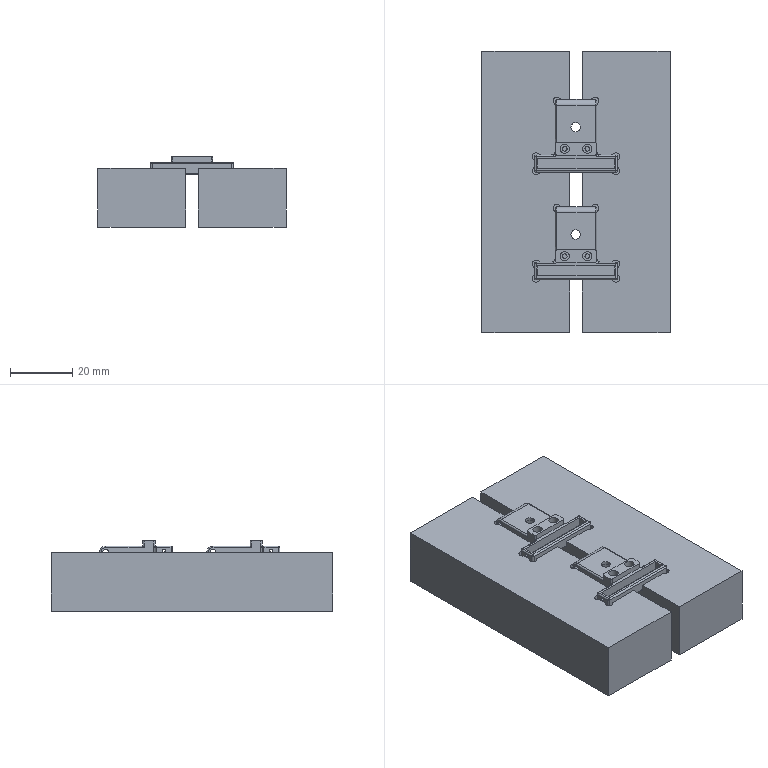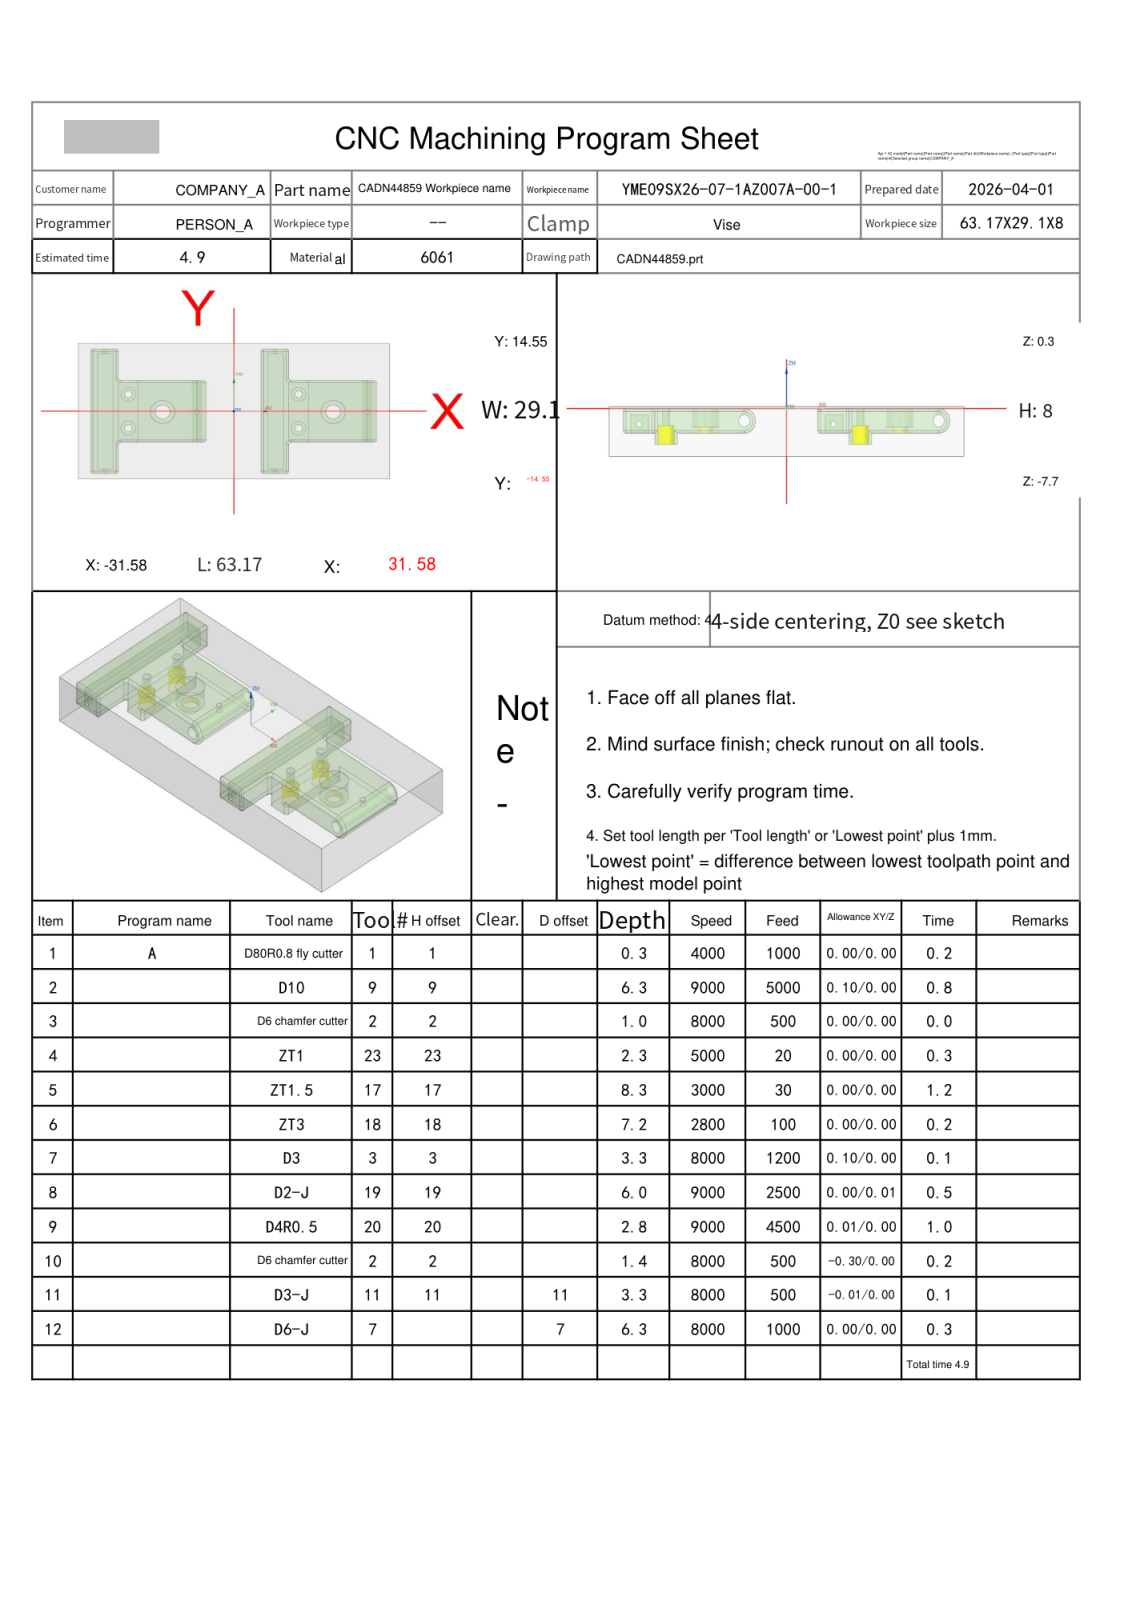NC program | NX | posted by the shop | part box 60.696 x 90.669 x 22.754 mm
Lines 2495 to 3978 of 3978:
N9 T20 M06
(D4R0.5  D=4. R=0.5 H=20 ce=0.01 di=0.00)
G00 G90 G54 X-3.173 Y-7.756 M03 S9000
G43 H20 Z10.3
M08
Z.484
G01 Z-.016 F4500.
X-6.415 Y-7.798
X-7.496 Y-7.812
X-7.515 Y-7.821
X-22.266
Y-12.848
G02 X-23.952 Y-14.535 I-1.687 J0.0
G01 X-28.584
G02 X-30.271 Y-12.848 I0.0 J1.687
G01 Y12.848
G02 X-28.584 Y14.535 I1.687 J0.0
G01 X-23.952
G02 X-22.266 Y12.848 I0.0 J-1.687
G01 Y7.821
X-7.515
X-7.496 Y7.812
X-6.415 Y7.798
Y7.852 Z-.028
Y7.904 Z-.04
X-7.515 Y7.925
X-22.162
Y12.848
G03 X-23.952 Y14.639 I-1.791 J0.0
G01 X-28.584
G03 X-30.375 Y12.848 I0.0 J-1.791
G01 Y-12.848
G03 X-28.584 Y-14.639 I1.791 J0.0
G01 X-23.952
G03 X-22.162 Y-12.848 I0.0 J1.791
G01 Y-7.925
X-7.515
X-6.415 Y-7.904
Y-7.963 Z-.057
Y-8.002 Z-.074
X-7.496 Y-8.013
X-7.515 Y-8.02
X-22.066
Y-12.848
G02 X-23.952 Y-14.734 I-1.886 J0.0
G01 X-28.584
G02 X-30.471 Y-12.848 I0.0 J1.886
G01 Y12.848
G02 X-28.584 Y14.734 I1.886 J0.0
G01 X-23.952
G02 X-22.066 Y12.848 I0.0 J-1.886
G01 Y8.02
X-7.515
X-7.496 Y8.013
X-6.415 Y8.002
Y8.055 Z-.095
Y8.101 Z-.116
X-7.496 Y8.106
X-7.515 Y8.112
X-21.974
Y12.848
G03 X-23.952 Y14.826 I-1.978 J0.0
G01 X-28.584
G03 X-30.562 Y12.848 I0.0 J-1.978
G01 Y-12.848
G03 X-28.584 Y-14.826 I1.978 J0.0
G01 X-23.952
G03 X-21.974 Y-12.848 I0.0 J1.978
G01 Y-8.112
X-7.515
X-7.496 Y-8.106
X-6.415 Y-8.101
Y-8.151 Z-.142
X-6.416 Y-8.191 Z-.168
X-7.496 Y-8.196
X-7.515 Y-8.198
X-21.888
Y-12.848
G02 X-23.952 Y-14.913 I-2.065 J0.0
G01 X-28.584
G02 X-30.649 Y-12.848 I0.0 J2.065
G01 Y12.848
G02 X-28.584 Y14.913 I2.065 J0.0
G01 X-23.952
G02 X-21.888 Y12.848 I0.0 J-2.065
G01 Y8.198
X-7.515
X-7.496 Y8.196
X-6.416 Y8.191
X-6.415 Y8.236 Z-.198
Y8.273 Z-.228
X-7.496
X-7.515 Y8.279
X-21.807
Y12.848
G03 X-23.952 Y14.994 I-2.146 J0.0
G01 X-28.584
G03 X-30.73 Y12.848 I0.0 J-2.146
G01 Y-12.848
G03 X-28.584 Y-14.994 I2.146 J0.0
G01 X-23.952
G03 X-21.807 Y-12.848 I0.0 J2.146
G01 Y-8.279
X-7.515
X-7.496 Y-8.273
X-6.415
Y-8.31 Z-.262
Y-8.351 Z-.296
X-7.515 Y-8.354
X-21.732
Y-12.848
G02 X-23.952 Y-15.068 I-2.22 J0.0
G01 X-28.584
G02 X-30.804 Y-12.848 I0.0 J2.22
G01 Y12.848
G02 X-28.584 Y15.068 I2.22 J0.0
G01 X-23.952
G02 X-21.732 Y12.848 I0.0 J-2.22
G01 Y8.354
X-7.515
X-6.415 Y8.351
Y8.385 Z-.333
X-6.416 Y8.415 Z-.37
X-7.496 Y8.412
X-7.515 Y8.421
X-21.665
Y12.848
G03 X-23.952 Y15.135 I-2.287 J0.0
G01 X-28.584
G03 X-30.871 Y12.848 I0.0 J-2.287
G01 Y-12.848
G03 X-28.584 Y-15.135 I2.287 J0.0
G01 X-23.952
G03 X-21.665 Y-12.848 I0.0 J2.287
G01 Y-8.421
X-7.515
X-7.496 Y-8.412
X-6.416 Y-8.415
X-6.415 Y-8.448 Z-.411
Y-8.476 Z-.451
X-7.496
X-7.515 Y-8.48
X-21.606
Y-12.848
G02 X-23.952 Y-15.194 I-2.346 J0.0
G01 X-28.584
G02 X-30.931 Y-12.848 I0.0 J2.346
G01 Y12.848
G02 X-28.584 Y15.194 I2.346 J0.0
G01 X-23.952
G02 X-21.606 Y12.848 I0.0 J-2.346
G01 Y8.48
X-7.515
X-7.496 Y8.476
X-6.415
Y8.5 Z-.495
Y8.526 Z-.538
X-7.496 Y8.527
X-7.515 Y8.531
X-21.556
Y12.848
G03 X-23.952 Y15.245 I-2.397 J0.0
G01 X-28.584
G03 X-30.981 Y12.848 I0.0 J-2.397
G01 Y-12.848
G03 X-28.584 Y-15.245 I2.397 J0.0
G01 X-23.952
G03 X-21.556 Y-12.848 I0.0 J2.397
G01 Y-8.531
X-7.515
X-7.496 Y-8.527
X-6.424 Y-8.525
Y-8.544 Z-.583
Y-8.57 Z-.629
X-7.515 Y-8.572
X-21.514
Y-12.848
G02 X-23.952 Y-15.287 I-2.439 J0.0
G01 X-28.584
G02 X-31.023 Y-12.848 I0.0 J2.439
G01 Y12.848
G02 X-28.584 Y15.287 I2.439 J0.0
G01 X-23.952
G02 X-21.514 Y12.848 I0.0 J-2.439
G01 Y8.572
X-7.515
X-6.415 Y8.567
Y8.586 Z-.675
Y8.599 Z-.722
X-7.515 Y8.604
X-21.482
Y12.848
G03 X-23.952 Y15.318 I-2.47 J0.0
G01 X-28.584
G03 X-31.055 Y12.848 I0.0 J-2.47
G01 Y-12.848
G03 X-28.584 Y-15.318 I2.47 J0.0
G01 X-23.952
G03 X-21.482 Y-12.848 I0.0 J2.47
G01 Y-8.604
X-7.515
X-6.424 Y-8.6
Y-8.613 Z-.768
Y-8.625 Z-.814
X-7.515 Y-8.626
X-21.46
Y-12.848
G02 X-23.952 Y-15.341 I-2.493 J0.0
G01 X-28.584
G02 X-31.077 Y-12.848 I0.0 J2.493
G01 Y12.848
G02 X-28.584 Y15.341 I2.493 J0.0
G01 X-23.952
G02 X-21.46 Y12.848 I0.0 J-2.493
G01 Y8.626
X-7.515
X-6.424 Y8.622
Y8.629 Z-.861
Y8.634 Z-.907
X-6.433 Y8.633
X-7.496 Y8.636
X-7.515 Y8.64
X-21.447
Y12.848
G03 X-23.952 Y15.354 I-2.506 J0.0
G01 X-28.584
G03 X-31.09 Y12.848 I0.0 J-2.506
G01 Y-12.848
G03 X-28.584 Y-15.354 I2.506 J0.0
G01 X-23.952
G03 X-21.447 Y-12.848 I0.0 J2.506
G01 Y-8.64
X-7.515
X-7.496 Y-8.636
X-6.424 Y-8.635
Y-8.643 Z-1.
X-7.515 Y-8.644
X-21.387
X-21.442
Y-8.779
Y-12.858
X-21.446 Y-12.978
G02 X-23.655 Y-15.34 I-2.507 J.13
G01 X-23.952 Y-15.358
X-28.595 Y-15.357
X-28.724 Y-15.354
G02 X-31.094 Y-12.848 I.139 J2.506
G01 Y12.858
X-31.088 Y13.027
G02 X-28.724 Y15.354 I2.504 J-.179
G01 X-28.585 Y15.358
X-23.952
X-23.655 Y15.34
G02 X-21.442 Y12.848 I-.297 J-2.492
G01 Y8.779
Y8.644
X-21.387
X-7.515
X-6.424 Y8.643
G00 Z10.3
X31.436 Y-7.732
Z.484
G01 Z-.016
X28.185 Y-7.798
X27.085 Y-7.821
X12.334
Y-12.848
G02 X10.648 Y-14.535 I-1.687 J0.0
G01 X6.016
G02 X4.329 Y-12.848 I0.0 J1.687
G01 Y12.848
G02 X6.016 Y14.535 I1.687 J0.0
G01 X10.648
G02 X12.334 Y12.848 I0.0 J-1.687
G01 Y7.821
X27.085
X28.185 Y7.798
Y7.852 Z-.028
Y7.904 Z-.04
X27.085 Y7.925
X12.438
Y12.848
G03 X10.648 Y14.639 I-1.791 J0.0
G01 X6.016
G03 X4.225 Y12.848 I0.0 J-1.791
G01 Y-12.848
G03 X6.016 Y-14.639 I1.791 J0.0
G01 X10.648
G03 X12.438 Y-12.848 I0.0 J1.791
G01 Y-7.925
X27.085
X28.185 Y-7.904
Y-7.962 Z-.057
Y-8.003 Z-.074
X27.085 Y-8.02
X12.534
Y-12.848
G02 X10.648 Y-14.734 I-1.886 J0.0
G01 X6.016
G02 X4.129 Y-12.848 I0.0 J1.886
G01 Y12.848
G02 X6.016 Y14.734 I1.886 J0.0
G01 X10.648
G02 X12.534 Y12.848 I0.0 J-1.886
G01 Y8.02
X27.085
X28.185 Y8.003
Y8.055 Z-.095
Y8.101 Z-.116
X27.085 Y8.112
X12.626
Y12.848
G03 X10.648 Y14.826 I-1.978 J0.0
G01 X6.016
G03 X4.038 Y12.848 I0.0 J-1.978
G01 Y-12.848
G03 X6.016 Y-14.826 I1.978 J0.0
G01 X10.648
G03 X12.626 Y-12.848 I0.0 J1.978
G01 Y-8.112
X27.085
X28.185 Y-8.101
Y-8.148 Z-.142
Y-8.191 Z-.168
X27.085 Y-8.198
X12.712
Y-12.848
G02 X10.648 Y-14.913 I-2.065 J0.0
G01 X6.016
G02 X3.951 Y-12.848 I0.0 J2.065
G01 Y12.848
G02 X6.016 Y14.913 I2.065 J0.0
G01 X10.648
G02 X12.712 Y12.848 I0.0 J-2.065
G01 Y8.198
X27.085
X28.185 Y8.191
Y8.236 Z-.198
X28.184 Y8.272 Z-.228
X27.085 Y8.279
X12.793
Y12.848
G03 X10.648 Y14.994 I-2.146 J0.0
G01 X6.016
G03 X3.87 Y12.848 I0.0 J-2.146
G01 Y-12.848
G03 X6.016 Y-14.994 I2.146 J0.0
G01 X10.648
G03 X12.793 Y-12.848 I0.0 J2.146
G01 Y-8.279
X27.085
X28.184 Y-8.272
Y-8.314 Z-.262
Y-8.347 Z-.296
X28.154 Y-8.346
X27.085 Y-8.354
X12.868
Y-12.848
G02 X10.648 Y-15.068 I-2.22 J0.0
G01 X6.016
G02 X3.796 Y-12.848 I0.0 J2.22
G01 Y12.848
G02 X6.016 Y15.068 I2.22 J0.0
G01 X10.648
G02 X12.868 Y12.848 I0.0 J-2.22
G01 Y8.354
X27.085
X28.154 Y8.346
X28.184 Y8.347
Y8.381 Z-.333
Y8.415 Z-.37
X28.131
G02 X27.085 Y8.421 I0.0 J88.093
G01 X12.935
Y12.848
G03 X10.648 Y15.135 I-2.287 J0.0
G01 X6.016
G03 X3.729 Y12.848 I0.0 J-2.287
G01 Y-12.848
G03 X6.016 Y-15.135 I2.287 J0.0
G01 X10.648
G03 X12.935 Y-12.848 I0.0 J2.287
G01 Y-8.421
X27.085
G02 X27.747 Y-8.41 I.663 J-20.048
X28.184 Y-8.415 I0.0 J-20.059
G01 Y-8.445 Z-.411
Y-8.474 Z-.451
X27.085 Y-8.48
X12.994
Y-12.848
G02 X10.648 Y-15.194 I-2.346 J0.0
G01 X6.016
G02 X3.669 Y-12.848 I0.0 J2.346
G01 Y12.848
G02 X6.016 Y15.194 I2.346 J0.0
G01 X10.648
G02 X12.994 Y12.848 I0.0 J-2.346
G01 Y8.48
X27.085
X28.184 Y8.474
Y8.5 Z-.495
Y8.526 Z-.538
X27.085 Y8.531
X13.044
Y12.848
G03 X10.648 Y15.245 I-2.397 J0.0
G01 X6.016
G03 X3.619 Y12.848 I0.0 J-2.397
G01 Y-12.848
G03 X6.016 Y-15.245 I2.397 J0.0
G01 X10.648
G03 X13.044 Y-12.848 I0.0 J2.397
G01 Y-8.531
X27.085
X28.181 Y-8.525
Y-8.544 Z-.583
Y-8.57 Z-.629
X27.085 Y-8.572
X13.086
Y-12.848
G02 X10.648 Y-15.287 I-2.439 J0.0
G01 X6.016
G02 X3.577 Y-12.848 I0.0 J2.439
G01 Y12.848
G02 X6.016 Y15.287 I2.439 J0.0
G01 X10.648
G02 X13.086 Y12.848 I0.0 J-2.439
G01 Y8.572
X27.085
X28.184 Y8.567
Y8.586 Z-.675
Y8.599 Z-.722
X27.085 Y8.604
X13.118
Y12.848
G03 X10.648 Y15.318 I-2.47 J0.0
G01 X6.016
G03 X3.545 Y12.848 I0.0 J-2.47
G01 Y-12.848
G03 X6.016 Y-15.318 I2.47 J0.0
G01 X10.648
G03 X13.118 Y-12.848 I0.0 J2.47
G01 Y-8.604
X27.085
X28.181 Y-8.6
Y-8.613 Z-.768
Y-8.625 Z-.814
X27.085 Y-8.626
X13.14
Y-12.848
G02 X10.648 Y-15.341 I-2.493 J0.0
G01 X6.016
G02 X3.523 Y-12.848 I0.0 J2.493
G01 Y12.848
G02 X6.016 Y15.341 I2.493 J0.0
G01 X10.648
G02 X13.14 Y12.848 I0.0 J-2.493
G01 Y8.626
X27.085
X28.181 Y8.622
Y8.629 Z-.861
Y8.634 Z-.907
X28.172 Y8.633
X27.085 Y8.64
X13.153
Y12.848
G03 X10.648 Y15.354 I-2.506 J0.0
G01 X6.016
G03 X3.51 Y12.848 I0.0 J-2.506
G01 Y-12.848
G03 X6.016 Y-15.354 I2.506 J0.0
G01 X10.648
G03 X13.153 Y-12.848 I0.0 J2.506
G01 Y-8.64
X27.085
X28.181 Y-8.635
Y-8.643 Z-1.
X27.085 Y-8.644
X13.158
Y-12.848
G02 X10.804 Y-15.353 I-2.51 J0.0
G01 X10.648 Y-15.358
X6.015
X5.864 Y-15.353
G02 X3.509 Y-12.974 I.152 J2.505
G01 X3.506 Y-12.848
X3.507 Y12.858
X3.509 Y12.974
G02 X5.391 Y15.279 I2.507 J-.126
G01 X5.449 Y15.293
X5.68 Y15.335
X5.7 Y15.338
X5.864 Y15.353
X6.015 Y15.358
X10.648
X10.804 Y15.353
G02 X13.158 Y12.848 I-.156 J-2.505
G01 Y8.644
X27.085
X28.181 Y8.643
G00 Z10.3
G00 G90 X23.972 Y9.673 M03 S9000
Z10.3
Z.491
G01 Z-.009 F4500.
G03 X25.972 Y7.673 I2. J0.0
G02 X26.537 Y7.748 I.565 J-2.104
X28.641 Y6.134 I0.0 J-2.178
G01 Y-6.134
G02 X26.537 Y-7.748 I-2.104 J.565
X25.972 Y-7.673 I0.0 J2.178
G01 Y-7.815 Z-.015
Y-7.847 Z-.021
X27.135 Y-7.833
G03 X28.916 Y-6.134 I-.022 J1.806
G01 Y6.134
G03 X27.135 Y7.833 I-1.803 J-.107
G01 X25.972 Y7.847
Y7.883 Z-.029
Y7.898 Z-.037
X27.347 Y7.868
X27.555 Y7.824
G02 X28.999 Y6.134 I-.377 J-1.784
G01 Y-6.134
G02 X27.555 Y-7.824 I-1.821 J.094
G01 X27.347 Y-7.868
X25.972 Y-7.898
Y-7.947 Z-.047
Y-7.977 Z-.057
X27.263 Y-7.952
G03 X29.126 Y-6.134 I-.038 J1.903
G01 Y6.134
G03 X27.263 Y7.952 I-1.901 J-.085
G01 X25.972 Y7.977
Y8.01 Z-.069
Y8.039 Z-.081
X27.347 Y8.013
X27.63 Y7.966
G02 X29.227 Y6.134 I-.373 J-1.937
G01 Y-6.134
G02 X27.63 Y-7.966 I-1.969 J.105
G01 X27.347 Y-8.013
X25.972 Y-8.039
Y-8.07 Z-.095
Y-8.098 Z-.109
X27.347 Y-8.076
X27.566 Y-8.044
G03 X29.326 Y-6.134 I-.291 J2.033
G01 Y6.134
G03 X27.566 Y8.044 I-2.05 J-.122
G01 X27.347 Y8.076
X25.972 Y8.098
Y8.128 Z-.125
Y8.156 Z-.141
G02 X26.507 Y8.177 I.535 J-6.848
X27.805 Y8.053 I0.0 J-6.869
X29.422 Y6.134 I-.441 J-2.013
G01 Y-6.134
G02 X27.805 Y-8.053 I-2.058 J.093
X26.507 Y-8.177 I-1.298 J6.746
X25.972 Y-8.156 I0.0 J6.869
G01 Y-8.185 Z-.159
Y-8.211 Z-.177
X27.347 Y-8.197
X27.63 Y-8.155
G03 X29.518 Y-6.134 I-.298 J2.17
G01 Y6.134
G03 X27.63 Y8.155 I-2.185 J-.148
G01 X27.347 Y8.197
X25.972 Y8.211
Y8.239 Z-.196
Y8.265 Z-.216
X27.347 Y8.245
X27.551 Y8.222
G02 X29.052 Y7.488 I-.281 J-2.475
X29.611 Y6.134 I-1.568 J-1.439
G01 Y-6.134
G02 X28.48 Y-7.926 I-2.113 J.08
X27.11 Y-8.258 I-1.37 J2.66
G01 X27.064
X25.986
X25.972 Y-8.265
Y-8.291 Z-.237
Y-8.315 Z-.259
X27.245 Y-8.3
G03 X28.759 Y-7.832 I-.034 J2.79
X29.702 Y-6.134 I-1.176 J1.764
G01 Y6.139
G03 X29.364 Y7.219 I-1.892 J0.0
X27.63 Y8.264 I-2.033 J-1.413
G01 X27.347 Y8.299
X25.972 Y8.315
Y8.34 Z-.282
Y8.363 Z-.305
X27.347 Y8.349
X27.63 Y8.318
G02 X29.33 Y7.401 I-.3 J-2.588
X29.792 Y6.134 I-1.523 J-1.273
G01 Y-6.134
G02 X28.51 Y-8.053 I-2.204 J.084
X27.107 Y-8.359 I-1.403 J3.067
G01 X27.064
X25.986
X25.972 Y-8.363
Y-8.386 Z-.33
Y-8.408 Z-.355
X27.246 Y-8.392
G03 X28.76 Y-7.984 I-.04 J3.156
X29.879 Y-6.134 I-1.085 J1.92
G01 Y6.134
G03 X29.047 Y7.788 I-2.19 J-.065
X27.347 Y8.391 I-1.796 J-2.367
G01 X25.972 Y8.408
Y8.43 Z-.382
Y8.45 Z-.409
X27.347 Y8.435
X27.63 Y8.406
G02 X29.047 Y7.875 I-.296 J-2.94
X29.964 Y6.134 I-1.312 J-1.804
G01 Y-6.134
G02 X29.047 Y-7.875 I-2.23 J.063
X27.63 Y-8.406 I-1.712 J2.408
G01 X27.347 Y-8.435
X25.972 Y-8.45
Y-8.47 Z-.437
X25.973 Y-8.489 Z-.465
X27.347 Y-8.481
X27.63 Y-8.452
G03 X29.047 Y-7.95 I-.321 J3.157
X30.047 Y-6.134 I-1.248 J1.872
G01 Y6.134
G03 X29.047 Y7.95 I-2.249 J-.056
X27.63 Y8.452 I-1.738 J-2.656
G01 X27.347 Y8.481
X25.973 Y8.489
Y8.507 Z-.495
Y8.524 Z-.525
X27.347 Y8.514
X27.63 Y8.492
G02 X29.047 Y8.018 I-.296 J-3.237
X30.128 Y6.134 I-1.198 J-1.94
G01 Y-6.134
G02 X29.047 Y-8.018 I-2.279 J.056
X27.63 Y-8.492 I-1.712 J2.763
X26.493 Y-8.533 I-1.138 J15.871
X25.973 Y-8.524 I0.0 J15.911
G01 Y-8.54 Z-.557
Y-8.555 Z-.589
X27.347 Y-8.548
X27.63 Y-8.525
G03 X29.047 Y-8.082 I-.268 J3.342
X30.206 Y-6.134 I-1.149 J2.003
G01 Y6.134
G03 X29.047 Y8.082 I-2.309 J-.055
X27.63 Y8.525 I-1.684 J-2.899
G01 X27.347 Y8.548
X25.973 Y8.555
Y8.582 Z-.655
X25.987 Y8.576
X27.347 Y8.571
X27.63 Y8.555
G02 X29.047 Y8.143 I-.237 J-3.451
X30.281 Y6.134 I-1.112 J-2.067
G01 Y-6.134
G02 X29.047 Y-8.143 I-2.346 J.058
X27.63 Y-8.555 I-1.653 J3.038
G01 X27.347 Y-8.571
X25.987 Y-8.576
X25.973 Y-8.582
Y-8.594 Z-.689
Y-8.605 Z-.724
G03 X26.441 Y-8.61 I.468 J21.709
X27.63 Y-8.577 I0.0 J21.714
X29.047 Y-8.203 I-.173 J3.518
X30.354 Y-6.134 I-1.077 J2.128
G01 Y6.134
G03 X29.047 Y8.203 I-2.384 J-.059
X27.63 Y8.577 I-1.589 J-3.143
G01 X27.347 Y8.594
X25.973 Y8.605
X25.984 Y8.623 Z-.796
X27.352 Y8.618
X27.63 Y8.601
G02 X28.859 Y8.336 I-.17 J-3.771
X30.424 Y6.134 I-.869 J-2.274
G01 Y-6.134
G02 X28.859 Y-8.336 I-2.434 J.073
X27.63 Y-8.601 I-1.399 J3.506
G01 X27.352 Y-8.618
X25.984 Y-8.623
Y-8.635 Z-.871
X26.002 Y-8.63
X27.272
G03 X28.213 Y-8.555 I0.0 J5.964
X29.33 Y-8.141 I-.481 J3.007
G01 X29.471 Y-8.053
G03 X30.491 Y-6.134 I-1.377 J1.962
G01 Y6.134
G03 X30.041 Y7.488 I-2.364 J-.034
X28.674 Y8.443 I-2.109 J-1.564
X27.394 Y8.628 I-1.28 J-4.339
G01 X27.347 Y8.627
X26.002 Y8.63
X25.984 Y8.635
Y8.642 Z-.948
X27.347 Y8.636
X27.63 Y8.629
G02 X28.763 Y8.449 I-.065 J-4.068
X30.286 Y7.205 I-.762 J-2.488
X30.554 Y6.134 I-2.188 J-1.116
G01 Y-6.134
G02 X29.876 Y-7.771 I-2.394 J.034
X28.48 Y-8.526 I-1.964 J1.96
X27.898 Y-8.618 I-1.417 J7.085
X26.45 Y-8.645 I-1.448 J38.753
X25.984 Y-8.642 I0.0 J38.78
G01 X25.993 Y-8.644 Z-1.028
G03 X26.566 Y-8.648 I.573 J39.735
X27.914 Y-8.625 I0.0 J39.739
X29.625 Y-8.053 I-.089 J3.114
X30.615 Y-6.134 I-1.434 J1.954
G01 Y6.134
G03 X29.625 Y8.053 I-2.423 J-.035
X27.914 Y8.625 I-1.801 J-2.542
X26.678 Y8.652 I-1.235 J-28.393
X25.993 Y8.644 I0.0 J-28.42
G01 Z-1.11
X27.63
X28.022 Y8.629
G02 X29.613 Y8.113 I-.121 J-3.087
X30.672 Y6.134 I-1.395 J-2.02
G01 Y-6.134
G02 X29.613 Y-8.113 I-2.454 J.04
X28.023 Y-8.628 I-1.711 J2.57
G01 X27.63 Y-8.644
X25.993
Z-1.194
X27.63
X27.914 Y-8.641
G03 X29.304 Y-8.336 I0.0 J3.322
X30.726 Y-6.134 I-1.059 J2.244
G01 Y6.134
G03 X29.304 Y8.336 I-2.481 J-.042
X27.914 Y8.641 I-1.391 J-3.018
G01 X27.63 Y8.644
X25.993
Z-1.281
X27.914
X28.197 Y8.631
G02 X29.613 Y8.198 I-.099 J-2.86
X30.777 Y6.134 I-1.315 J-2.102
G01 Y-6.134
G02 X29.047 Y-8.471 I-2.517 J.054
X27.95 Y-8.644 I-1.096 J3.395
G01 X27.914
X25.993
Z-1.369
X28.033
G03 X29.059 Y-8.487 I0.0 J3.444
X30.766 Y-6.64 I-.752 J2.407
X30.824 Y-6.134 I-5.478 J.882
G01 Y6.134
G03 X30.766 Y6.64 I-5.536 J-.375
X29.613 Y8.235 I-2.436 J-.547
X28.197 Y8.637 I-1.472 J-2.488
G01 X27.914 Y8.644
X25.993
Z-1.459
X28.197
G02 X29.33 Y8.408 I-.03 J-2.989
X30.867 Y6.134 I-.963 J-2.308
G01 Y-6.134
G02 X29.33 Y-8.408 I-2.501 J.034
X28.197 Y-8.644 I-1.163 J2.754
G01 X25.993
Z-1.551
X28.197
X28.218
G03 X29.33 Y-8.435 I0.0 J3.061
X30.907 Y-6.134 I-.939 J2.335
G01 Y6.134
G03 X29.33 Y8.435 I-2.516 J-.034
X28.218 Y8.644 I-1.112 J-2.852
G01 X28.197
X25.993
Z-1.644
X28.197
X28.48 Y8.632
G02 X30.694 Y7.205 I-.091 J-2.573
X30.943 Y6.134 I-2.386 J-1.119
G01 Y-6.134
G02 X29.33 Y-8.453 I-2.508 J.023
X28.266 Y-8.645 I-1.063 J2.862
G01 X28.197 Y-8.644
X25.993
Z-1.739
X28.197
X28.48 Y-8.637
G03 X30.976 Y-6.134 I-.04 J2.535
G01 Y6.134
G03 X28.48 Y8.637 I-2.535 J-.032
G01 X28.197 Y8.644
X25.993
Z-1.835
X28.197
X28.48 Y8.641
G02 X31.004 Y6.134 I-.012 J-2.537
G01 Y-6.134
G02 X28.48 Y-8.641 I-2.537 J.029
G01 X28.197 Y-8.644
X25.993
Z-1.932
X28.48
X28.493
G03 X31.029 Y-6.134 I0.0 J2.536
G01 Y6.134
G03 X28.493 Y8.644 I-2.536 J-.026
G01 X28.48
X25.993
Z-2.03
X28.48
X28.507
G02 X30.805 Y7.205 I0.0 J-2.555
X31.05 Y6.134 I-2.318 J-1.093
G01 Y-6.134
G02 X28.864 Y-8.618 I-2.527 J.02
G01 X28.48 Y-8.644
X25.993
Z-2.128
X28.48
X28.534
G03 X31.067 Y-6.134 I0.0 J2.533
G01 Y6.134
G03 X28.534 Y8.644 I-2.533 J-.022
G01 X28.48
X25.993
Z-2.221
X28.48
X28.548 Y8.645
G02 X31.026 Y6.64 I0.0 J-2.534
X31.079 Y6.134 I-5.456 J-.825
G01 Y-6.134
G02 X31.026 Y-6.64 I-5.546 J.323
X28.548 Y-8.645 I-2.478 J.529
G01 X28.48 Y-8.644
X25.993
Z-2.314
X28.48
X28.55 Y-8.645
G03 X30.687 Y-7.488 I0.0 J2.552
X31.088 Y-6.134 I-2.235 J1.397
G01 Y6.134
G03 X31.033 Y6.64 I-5.686 J-.354
X28.763 Y8.635 I-2.467 J-.519
G01 X28.48 Y8.644
X25.993
Z-2.407
X28.48
X28.763 Y8.635
G02 X31.093 Y6.134 I-.188 J-2.511
G01 Y-6.134
G02 X28.763 Y-8.635 I-2.518 J.01
G01 X28.48 Y-8.644
X25.993
Z-2.5
X28.583
G03 X31.079 Y-6.386 I0.0 J2.509
X31.094 Y-6.08 I-3.046 J.306
G01 Y5.793
Y6.125
G03 X28.576 Y8.644 I-2.519 J0.0
G01 X25.993
G00 Z10.3
X-10.632 Y9.673
Z.491
G01 Z-.009
G03 X-8.632 Y7.673 I2. J0.0
G02 X-8.065 Y7.748 I.567 J-2.106
X-5.959 Y6.134 I0.0 J-2.181
G01 Y-6.135
G02 X-7.467 Y-7.643 I-1.508 J0.0
G01 X-7.476
X-8.48 Y-7.637
X-8.632 Y-7.673
Y-7.815 Z-.015
Y-7.847 Z-.021
X-8.48 Y-7.834
X-7.463 Y-7.828
G03 X-5.684 Y-6.134 I-.011 J1.793
G01 Y6.134
G03 X-7.211 Y7.803 I-1.801 J-.114
G01 X-7.366 Y7.827
X-8.632 Y7.847
Y7.883 Z-.029
Y7.898 Z-.037
G02 X-8.13 Y7.919 I.502 J-6.078
X-6.987 Y7.811 I0.0 J-6.099
X-5.601 Y6.136 I-.32 J-1.675
G01 Y-6.134
G02 X-6.989 Y-7.811 I-1.707 J0.0
X-8.13 Y-7.919 I-1.141 J5.991
X-8.632 Y-7.898 I0.0 J6.099
G01 Y-7.977 Z-.057
X-8.614 Y-7.969
X-7.366 Y-7.963
X-7.087 Y-7.923
G03 X-5.474 Y-6.134 I-.309 J1.901
G01 Y6.134
G03 X-7.087 Y7.923 I-1.922 J-.112
G01 X-7.366 Y7.963
X-8.614 Y7.969
X-8.632 Y7.977
Y8.01 Z-.069
Y8.039 Z-.081
X-7.366 Y8.028
X-7.087 Y7.988
G02 X-5.373 Y6.134 I-.262 J-1.962
G01 Y-6.134
G02 X-7.087 Y-7.988 I-1.976 J.108
G01 X-7.366 Y-8.028
X-8.632 Y-8.039
Y-8.07 Z-.095
Y-8.098 Z-.109
X-7.366 Y-8.087
X-7.056 Y-8.053
G03 X-5.274 Y-6.134 I-.266 J2.033
G01 Y6.134
G03 X-7.056 Y8.053 I-2.048 J-.114
G01 X-7.366 Y8.087
X-8.632 Y8.098
Y8.128 Z-.125
Y8.156 Z-.141
G02 X-8.128 Y8.173 I.504 J-7.622
X-6.922 Y8.077 I0.0 J-7.638
X-5.178 Y6.134 I-.328 J-2.048
G01 Y-6.134
G02 X-6.922 Y-8.077 I-2.072 J.105
X-8.128 Y-8.173 I-1.206 J7.543
X-8.632 Y-8.156 I0.0 J7.638
G01 Y-8.185 Z-.159
Y-8.211 Z-.177
X-8.614 Y-8.209
X-7.525
G03 X-6.237 Y-7.912 I0.0 J2.945
X-5.082 Y-6.134 I-.899 J1.848
G01 Y6.134
G03 X-5.27 Y6.923 I-2.016 J-.063
X-7.087 Y8.179 I-2.048 J-1.02
G01 X-7.366 Y8.204
X-8.632 Y8.211
Y8.239 Z-.196
Y8.265 Z-.216
G02 X-8.115 Y8.28 I.517 J-8.713
X-6.809 Y8.181 I0.0 J-8.729
X-4.989 Y6.134 I-.387 J-2.176
G01 Y-6.134
G02 X-6.809 Y-8.181 I-2.206 J.128
X-8.115 Y-8.28 I-1.307 J8.63
X-8.632 Y-8.265 I0.0 J8.729
G01 Y-8.291 Z-.237
Y-8.315 Z-.259
X-7.366 Y-8.305
X-7.087 Y-8.283
G03 X-5.363 Y-7.385 I-.266 J2.617
X-4.898 Y-6.135 I-1.447 J1.25
G01 Y6.134
G03 X-5.231 Y7.205 I-1.976 J-.027
X-6.903 Y8.248 I-1.991 J-1.331
X-8.12 Y8.329 I-1.217 J-9.064
X-8.632 Y8.315 I0.0 J-9.145
G01 Y8.34 Z-.282
Y8.363 Z-.305
X-8.614 Y8.359
X-7.366 Y8.354
X-7.162 Y8.341
G02 X-5.369 Y7.518 I-.172 J-2.736
X-4.808 Y6.137 I-1.418 J-1.381
G01 Y-6.134
G02 X-5.695 Y-7.814 I-2.154 J.063
G01 X-5.877 Y-7.925
G02 X-7.393 Y-8.354 I-1.526 J2.502
G01 X-8.614 Y-8.359
X-8.632 Y-8.363
Y-8.408 Z-.355
X-8.614 Y-8.4
X-7.366 Y-8.396
G03 X-5.953 Y-8.053 I-.054 J3.306
X-4.721 Y-6.134 I-1.005 J2.
G01 Y6.134
G03 X-5.533 Y7.771 I-2.168 J-.056
X-7.087 Y8.378 I-1.77 J-2.239
G01 X-7.366 Y8.396
X-8.614 Y8.4
X-8.632 Y8.408
Y8.45 Z-.409
X-8.614 Y8.445
X-7.366 Y8.44
X-7.087 Y8.42
G02 X-5.837 Y8.053 I-.254 J-3.174
X-4.636 Y6.134 I-1.038 J-1.986
G01 Y-6.134
G02 X-5.837 Y-8.053 I-2.24 J.066
X-7.087 Y-8.42 I-1.503 J2.807
G01 X-7.366 Y-8.44
X-8.614 Y-8.445
X-8.632 Y-8.45
Y-8.47 Z-.437
Y-8.489 Z-.465
X-7.366 Y-8.484
X-7.087 Y-8.466
G03 X-5.715 Y-8.053 I-.28 J3.422
X-4.553 Y-6.134 I-1.11 J1.983
G01 Y6.134
G03 X-5.715 Y8.053 I-2.272 J-.064
X-7.087 Y8.466 I-1.653 J-3.01
G01 X-7.366 Y8.484
X-8.632 Y8.489
Y8.507 Z-.495
Y8.524 Z-.525
X-7.366 Y8.517
X-7.087 Y8.502
G02 X-5.61 Y8.053 I-.205 J-3.331
X-4.472 Y6.134 I-1.147 J-1.976
G01 Y-6.134
G02 X-5.61 Y-8.053 I-2.284 J.057
X-7.087 Y-8.502 I-1.682 J2.883
G01 X-7.366 Y-8.517
X-8.632 Y-8.524
Y-8.54 Z-.557
Y-8.555 Z-.589
X-7.366 Y-8.55
X-7.087 Y-8.536
G03 X-5.504 Y-8.053 I-.18 J3.426
X-4.394 Y-6.134 I-1.193 J1.97
G01 Y6.134
G03 X-5.504 Y8.053 I-2.303 J-.051
X-7.087 Y8.536 I-1.763 J-2.944
G01 X-7.366 Y8.55
X-8.632 Y8.555
Y8.582 Z-.655
X-8.614 Y8.576
X-7.438
G02 X-6.241 Y8.426 I0.0 J-4.856
X-4.859 Y7.576 I-.671 J-2.638
X-4.319 Y6.134 I-1.797 J-1.496
G01 Y-6.134
G02 X-5.695 Y-8.219 I-2.367 J.065
X-7.087 Y-8.562 I-1.539 J3.248
G01 X-7.366 Y-8.573
X-8.614 Y-8.576
X-8.632 Y-8.582
Y-8.594 Z-.689
Y-8.605 Z-.724
G03 X-8.181 Y-8.61 I.451 J20.331
X-6.809 Y-8.564 I0.0 J20.336
X-5.416 Y-8.121 I-.279 J3.29
X-4.246 Y-6.134 I-1.192 J2.04
G01 Y6.134
G03 X-5.416 Y8.121 I-2.363 J-.053
X-6.809 Y8.564 I-1.672 J-2.848
X-8.181 Y8.61 I-1.372 J-20.29
X-8.632 Y8.605 I0.0 J-20.336
G01 X-8.619 Y8.623 Z-.796
X-7.276 Y8.618
X-7.087 Y8.61
G02 X-5.973 Y8.423 I-.18 J-4.498
X-4.449 Y7.205 I-.763 J-2.517
X-4.176 Y6.134 I-2.259 J-1.146
G01 Y-6.134
G02 X-5.138 Y-7.994 I-2.35 J.036
X-6.252 Y-8.499 I-1.71 J2.293
X-7.366 Y-8.62 I-1.149 J5.382
G01 X-8.602 Y-8.621
X-8.619 Y-8.623
Y-8.635 Z-.871
X-8.602 Y-8.63
X-7.644
X-7.223 Y-8.628
G03 X-6.53 Y-8.575 I-.023 J4.818
X-5.129 Y-8.053 I-.344 J3.065
X-4.109 Y-6.134 I-1.378 J1.963
G01 Y6.134
G03 X-4.38 Y7.205 I-2.53 J-.07
X-5.971 Y8.458 I-2.291 J-1.273
X-7.223 Y8.629 I-1.257 J-4.536
G01 X-8.602 Y8.63
X-8.619 Y8.635
Y8.642 Z-.948
X-7.087 Y8.633
X-6.809 Y8.623
G02 X-5.695 Y8.4 I-.195 J-3.875
X-4.311 Y7.205 I-.916 J-2.46
X-4.046 Y6.134 I-2.316 J-1.141
G01 Y-6.134
G02 X-5.051 Y-8.053 I-2.401 J.035
X-5.973 Y-8.489 I-1.653 J2.301
X-7.083 Y-8.633 I-1.11 J4.232
G01 X-7.087
X-7.366 Y-8.638
X-8.602 Y-8.64
X-8.619 Y-8.642
X-8.61 Y-8.644 Z-1.028
X-7.087 Y-8.642
X-6.809 Y-8.631
G03 X-5.416 Y-8.318 I-.059 J3.521
X-3.985 Y-6.134 I-1.037 J2.24
G01 Y6.134
G03 X-5.416 Y8.318 I-2.468 J-.056
X-6.809 Y8.631 I-1.452 J-3.208
G01 X-7.087 Y8.642
X-8.61 Y8.644
Z-1.11
X-6.809 Y8.639
X-6.53 Y8.624
G02 X-5.129 Y8.203 I-.158 J-3.064
X-3.928 Y6.134 I-1.242 J-2.105
G01 Y-6.134
G02 X-5.14 Y-8.209 I-2.444 J.036
X-6.666 Y-8.636 I-1.582 J2.712
G01 X-7.087 Y-8.644
X-8.61
Z-1.194
X-6.809
X-6.459 Y-8.628
G03 X-5.541 Y-8.433 I-.125 J2.842
G01 X-5.295 Y-8.336
G03 X-3.874 Y-6.134 I-1.061 J2.244
G01 Y6.134
G03 X-5.138 Y8.251 I-2.466 J-.036
X-6.53 Y8.632 I-1.483 J-2.686
G01 X-6.809 Y8.644
X-8.61
Z-1.281
X-6.809
X-6.53 Y8.639
G02 X-5.138 Y8.287 I-.035 J-3.075
X-3.88 Y6.64 I-1.185 J-2.208
X-3.823 Y6.134 I-5.921 J-.924
G01 Y-6.134
G02 X-5.229 Y-8.336 I-2.493 J.042
G01 X-5.416 Y-8.414
G02 X-6.53 Y-8.639 I-1.136 J2.762
G01 X-6.809 Y-8.644
X-8.61
Z-1.369
X-6.53
X-6.509
G03 X-5.138 Y-8.321 I0.0 J3.07
X-3.776 Y-6.134 I-1.129 J2.22
G01 Y6.134
G03 X-4.023 Y7.194 I-2.766 J-.087
X-5.166 Y8.336 I-2.292 J-1.152
X-6.512 Y8.644 I-1.346 J-2.785
G01 X-6.53
X-8.61
Z-1.459
X-6.53
X-6.252 Y8.632
G02 X-4.581 Y7.982 I-.106 J-2.745
X-3.733 Y6.134 I-1.679 J-1.889
G01 Y-6.134
G02 X-5.416 Y-8.467 I-2.508 J.035
X-6.467 Y-8.644 I-1.051 J3.031
G01 X-6.53
X-8.61
Z-1.551
X-6.53
X-6.252 Y-8.638
G03 X-5.138 Y-8.372 I-.055 J2.699
G01 X-5.061 Y-8.336
G03 X-3.693 Y-6.134 I-1.13 J2.228
G01 Y6.134
G03 X-3.746 Y6.64 I-6.085 J-.386
X-4.105 Y7.488 I-2.703 J-.644
X-6.252 Y8.638 I-2.186 J-1.502
G01 X-6.53 Y8.644
X-8.61
Z-1.644
X-6.252
G02 X-4.578 Y8.053 I-.02 J-2.722
X-3.657 Y6.134 I-1.618 J-1.958
G01 Y-6.134
G02 X-5.416 Y-8.507 I-2.524 J.033
X-6.252 Y-8.644 I-.887 J2.799
G01 X-8.61
Z-1.739
X-6.252
G03 X-5.416 Y-8.52 I-.003 J2.908
X-3.624 Y-6.134 I-.728 J2.412
G01 Y6.134
G03 X-4.032 Y7.488 I-2.554 J-.031
X-6.205 Y8.644 I-2.173 J-1.463
G01 X-6.252
X-8.61
Z-1.835
X-6.252
X-6.213
G02 X-5.416 Y8.532 I0.0 J-2.888
X-3.596 Y6.134 I-.697 J-2.419
G01 Y-6.134
G02 X-5.973 Y-8.629 I-2.522 J.023
G01 X-6.252 Y-8.644
X-8.61
Z-1.932
X-6.252
X-5.973 Y-8.633
G03 X-3.571 Y-6.134 I-.116 J2.516
G01 Y6.134
G03 X-5.973 Y8.633 I-2.519 J-.017
G01 X-6.252 Y8.644
X-8.61
Z-2.03
X-6.252
X-5.973 Y8.636
G02 X-3.55 Y6.134 I-.095 J-2.516
G01 Y-6.134
G02 X-5.973 Y-8.636 I-2.518 J.014
G01 X-6.252 Y-8.644
X-8.61
Z-2.128
X-6.252
X-5.973 Y-8.64
G03 X-3.533 Y-6.134 I-.085 J2.524
G01 Y6.134
G03 X-5.973 Y8.64 I-2.526 J-.018
G01 X-6.252 Y8.644
X-8.61
Z-2.221
X-6.252
X-5.973 Y8.643
G02 X-3.521 Y6.134 I-.075 J-2.526
G01 Y-6.134
X-3.527 Y-6.149
X-3.534 Y-6.358
G02 X-5.973 Y-8.643 I-2.514 J.239
G01 X-6.252 Y-8.644
X-8.61
Z-2.314
X-6.252
X-6.016 Y-8.643
G03 X-3.523 Y-6.231 I-.013 J2.508
G01 X-3.519 Y-6.149
X-3.512 Y-6.134
Y6.134
G03 X-5.973 Y8.643 I-2.526 J-.016
G01 X-6.252 Y8.644
X-8.61
Z-2.407
X-6.252
X-5.973 Y8.643
G02 X-3.507 Y6.134 I-.055 J-2.52
G01 Y-6.134
G02 X-5.973 Y-8.643 I-2.521 J.012
G01 X-6.252 Y-8.644
X-8.61
Z-2.5
X-6.252
X-6.002 Y-8.643
G03 X-3.522 Y-6.402 I-.013 J2.507
X-3.506 Y-6.084 I-2.983 J.319
G01 Y6.034
G03 X-3.526 Y6.415 I-3.487 J0.0
X-5.999 Y8.643 I-2.486 J-.273
G01 X-6.252 Y8.644
X-8.61
G00 Z10.3
G91 G28 Z0.0
M05
M09
G91 G28 Z0.0
M01
N10 T02 M06
(D6 chamfer cutter  D=6. R=0. H=02 ce=0.00 di=0.00)
G00 G90 G54 X-21.452 Y3.634 M03 S8000
G43 H02 Z20.
M08
G98 G81 X-21.452 Y3.634 Z-1.05 R3. F500.
Y-3.634
X13.148
Y3.634
G80
G00 Z20.
G00 G90 X-15.911 Y.905 M03 S8000
Z20.
Z2.5
G01 X-15.941 Y.868 Z2.483 F500.
X-16.078 Y.63 Z2.383
X-16.177 Y.375 Z2.283
X-16.237 Y.107 Z2.183
X-16.255 Y-.167 Z2.084
X-16.232 Y-.44 Z1.984
X-16.167 Y-.706 Z1.884
X-16.063 Y-.96 Z1.784
X-15.959 Y-1.14 Z1.708
X-15.792 Y-1.357 Z1.609
X-15.593 Y-1.546 Z1.509
X-15.368 Y-1.703 Z1.409
X-15.122 Y-1.824 Z1.309
X-14.86 Y-1.906 Z1.209
X-14.589 Y-1.948 Z1.11
X-14.315 Z1.01
X-14.044 Y-1.906 Z.91
X-13.783 Y-1.824 Z.81
X-13.536 Y-1.703 Z.71
X-13.312 Y-1.546 Z.611
X-13.113 Y-1.357 Z.511
X-12.945 Y-1.14 Z.411
X-12.841 Y-.96 Z.335
X-12.737 Y-.706 Z.235
X-12.673 Y-.44 Z.136
X-12.649 Y-.167 Z.036
X-12.668 Y.107 Z-.064
X-12.727 Y.375 Z-.164
X-12.827 Y.63 Z-.264
X-12.964 Y.868 Z-.363
X-13.135 Y1.082 Z-.463
X-13.337 Y1.267 Z-.563
X-13.565 Y1.42 Z-.663
X-13.814 Y1.536 Z-.763
X-14.077 Y1.613 Z-.862
X-14.348 Y1.65 Z-.962
X-14.452 Z-1.
G03 X-16.252 Y-.15 I0.0 J-1.8
X-14.452 Y-1.95 I1.8 J0.0
X-12.652 Y-.15 I0.0 J1.8
X-14.452 Y1.65 I-1.8 J0.0
X-14.946 Y1.581 I0.0 J-1.8
G01 Z1.5
G00 Z20.
X18.689 Y.905
Z2.5
G01 X18.659 Y.868 Z2.483
X18.522 Y.63 Z2.383
X18.423 Y.375 Z2.283
X18.363 Y.107 Z2.183
X18.345 Y-.167 Z2.084
X18.368 Y-.44 Z1.984
X18.433 Y-.706 Z1.884
X18.537 Y-.96 Z1.784
X18.641 Y-1.14 Z1.708
X18.808 Y-1.357 Z1.609
X19.007 Y-1.546 Z1.509
X19.232 Y-1.703 Z1.409
X19.478 Y-1.824 Z1.309
X19.74 Y-1.906 Z1.209
X20.011 Y-1.948 Z1.11
X20.285 Z1.01
X20.556 Y-1.906 Z.91
X20.817 Y-1.824 Z.81
X21.064 Y-1.703 Z.71
X21.288 Y-1.546 Z.611
X21.487 Y-1.357 Z.511
X21.655 Y-1.14 Z.411
X21.759 Y-.96 Z.335
X21.863 Y-.706 Z.235
X21.927 Y-.44 Z.136
X21.951 Y-.167 Z.036
X21.932 Y.107 Z-.064
X21.873 Y.375 Z-.164
X21.773 Y.63 Z-.264
X21.636 Y.868 Z-.363
X21.465 Y1.082 Z-.463
X21.263 Y1.267 Z-.563
X21.035 Y1.42 Z-.663
X20.786 Y1.536 Z-.763
X20.523 Y1.613 Z-.862
X20.252 Y1.65 Z-.962
X20.148 Z-1.
G03 X18.348 Y-.15 I0.0 J-1.8
X20.148 Y-1.95 I1.8 J0.0
X21.948 Y-.15 I0.0 J1.8
X20.148 Y1.65 I-1.8 J0.0
X19.654 Y1.581 I0.0 J-1.8
G01 Z1.5
G00 Z20.
G91 G28 Z0.0
M05
M09
G91 G28 Z0.0
M01
N11 T11 M06
(D3-J  D=3. R=0. H=11 ce=-0.01 di=0.00)
G00 G90 G54 X-14.902 Y-.283 M03 S8000
G43 H11 Z10.3
M08
Z-1.5
G01 Z-3. F500.
G41 D11
Y-.71
G03 X-14.452 Y-1.16 I.45 J0.0
X-13.442 Y-.15 I0.0 J1.01
X-14.452 Y.86 I-1.01 J0.0
X-15.462 Y-.15 I0.0 J-1.01
X-14.452 Y-1.16 I1.01 J0.0
X-14.063 Y-1.082 I0.0 J1.01
X-13.786 Y-.667 I-.174 J.415
G01 X-13.821 Y-.493
X-13.909 Y-.284
G40 X-13.986 Y-.099
Z-1.5
G00 Z10.3
X20.281 Y-.6
Z-1.5
G01 Z-3.
G41 D11
X20.708
G03 X21.158 Y-.15 I0.0 J.45
X20.148 Y.86 I-1.01 J0.0
X19.138 Y-.15 I0.0 J-1.01
X20.148 Y-1.16 I1.01 J0.0
X21.158 Y-.15 I0.0 J1.01
X21.08 Y.24 I-1.01 J0.0
X20.664 Y.516 I-.415 J-.174
G01 X20.491 Y.481
X20.282 Y.394
G40 X20.097 Y.317
Z-1.5
G00 Z10.3
G91 G28 Z0.0
M05
M09
G91 G28 Z0.0
M01
N12 T07 M06
(D6-J  D=6. R=0. H=00 ce=0.00 di=0.00)
G00 G90 G54 X1.428 Y-13.864 M03 S8000
G43 H00 Z20.
M08
Z-5.454
G01 Z-5.954 F1000.
G41 D07
X1.627 Y-13.842
G03 X2.516 Y-12.848 I-.111 J.994
G01 Y12.848
G02 X6.016 Y16.348 I3.5 J0.0
G01 X10.648
G02 X14.148 Y12.848 I0.0 J-3.5
G01 Y9.634
X28.584
G02 X32.084 Y6.134 I0.0 J-3.5
G01 Y-6.134
G02 X28.584 Y-9.634 I-3.5 J0.0
G01 X14.148
Y-12.848
G02 X10.648 Y-16.348 I-3.5 J0.0
G01 X6.016
G02 X2.516 Y-12.848 I0.0 J3.5
G01 Y-12.348
G03 X1.516 Y-11.348 I-1. J0.0
G01 G40 X1.316
Z-5.454
G00 Z20.
X-33.172 Y-13.864
Z-5.454
G01 Z-5.954
G41 D07
X-32.973 Y-13.842
G03 X-32.084 Y-12.848 I-.111 J.994
G01 Y12.848
G02 X-28.584 Y16.348 I3.5 J0.0
G01 X-23.952
G02 X-20.452 Y12.848 I0.0 J-3.5
G01 Y9.634
X-6.016
G02 X-2.516 Y6.134 I0.0 J-3.5
G01 Y-6.134
G02 X-6.016 Y-9.634 I-3.5 J0.0
G01 X-20.452
Y-12.848
G02 X-23.952 Y-16.348 I-3.5 J0.0
G01 X-28.584
G02 X-32.084 Y-12.848 I0.0 J3.5
G01 Y-12.348
G03 X-33.084 Y-11.348 I-1. J0.0
G01 G40 X-33.284
Z-5.454
G00 Z20.
M05
M09
G91 G28 Z0.0
G91 G28 Y0.0
M30
%